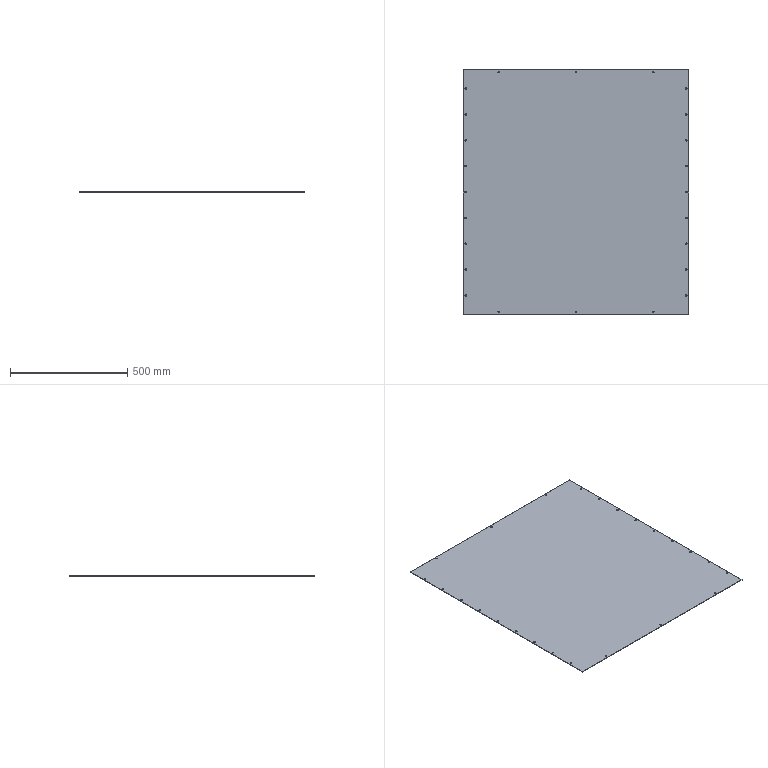Part | SolidWorks | 1 solid | 54 faces | box 962 x 1043 x 2 mm | volume 2005139 mm3 | cylinder 48 | plane 6 | commonest cylinder face diameters 6.5 x48